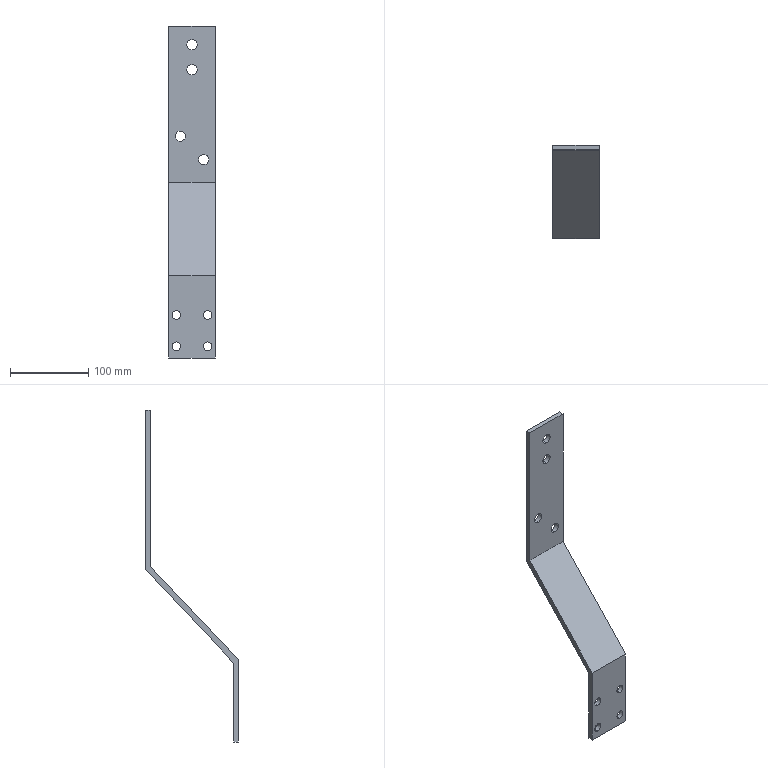Part | SolidWorks | features BaseBody 1 | 1 solid | 26 faces | box 60 x 119 x 425 mm | volume 174654 mm3 | cylinder 16 | plane 10 | commonest cylinder face diameters 11 x8 13 x8
STEP:
#1=CARTESIAN_POINT('',(546.946,-3258.473,957.471));
#2=VERTEX_POINT('',#1);
#3=CARTESIAN_POINT('',(546.946,-3258.473,944.471));
#4=VERTEX_POINT('',#3);
#5=CARTESIAN_POINT('',(546.946,-3258.473,950.971));
#6=DIRECTION('',(0.,-1.,0.));
#7=DIRECTION('',(0.,0.,-1.));
#8=AXIS2_PLACEMENT_3D('',#5,#6,#7);
#9=CIRCLE('',#8,6.5);
#10=EDGE_CURVE('',#2,#4,#9,.T.);
#11=ORIENTED_EDGE('',*,*,#10,.F.);
#12=CARTESIAN_POINT('',(546.946,-3264.473,957.471));
#13=VERTEX_POINT('',#12);
#14=CARTESIAN_POINT('',(546.946,-3307.534,957.471));
#15=DIRECTION('',(0.,-1.,0.));
#16=VECTOR('',#15,1000.);
#17=LINE('',#14,#16);
#18=EDGE_CURVE('',#2,#13,#17,.T.);
#19=ORIENTED_EDGE('',*,*,#18,.T.);
#20=CARTESIAN_POINT('',(546.946,-3264.473,944.471));
#21=VERTEX_POINT('',#20);
#22=CARTESIAN_POINT('',(546.946,-3264.473,950.971));
#23=DIRECTION('',(0.,1.,0.));
#24=DIRECTION('',(0.,0.,-1.));
#25=AXIS2_PLACEMENT_3D('',#22,#23,#24);
#26=CIRCLE('',#25,6.5);
#27=EDGE_CURVE('',#21,#13,#26,.T.);
#28=ORIENTED_EDGE('',*,*,#27,.F.);
#29=CARTESIAN_POINT('',(546.946,-3307.534,944.471));
#30=DIRECTION('',(0.,-1.,0.));
#31=VECTOR('',#30,1000.);
#32=LINE('',#29,#31);
#33=EDGE_CURVE('',#4,#21,#32,.T.);
#34=ORIENTED_EDGE('',*,*,#33,.F.);
#35=EDGE_LOOP('',(#11,#19,#28,#34));
#36=FACE_OUTER_BOUND('',#35,.T.);
#37=CARTESIAN_POINT('',(546.946,-3307.534,950.971));
#38=DIRECTION('',(0.,-1.,0.));
#39=DIRECTION('',(0.,0.,-1.));
#40=AXIS2_PLACEMENT_3D('',#37,#38,#39);
#41=CYLINDRICAL_SURFACE('',#40,6.5);
#42=ADVANCED_FACE('',(#36),#41,.F.);
#43=CARTESIAN_POINT('',(546.946,-3258.473,925.471));
#44=VERTEX_POINT('',#43);
#45=CARTESIAN_POINT('',(546.946,-3258.473,912.471));
#46=VERTEX_POINT('',#45);
#47=CARTESIAN_POINT('',(546.946,-3258.473,918.971));
#48=DIRECTION('',(0.,-1.,0.));
#49=DIRECTION('',(0.,0.,-1.));
#50=AXIS2_PLACEMENT_3D('',#47,#48,#49);
#51=CIRCLE('',#50,6.5);
#52=EDGE_CURVE('',#44,#46,#51,.T.);
#53=ORIENTED_EDGE('',*,*,#52,.F.);
#54=CARTESIAN_POINT('',(546.946,-3264.473,925.471));
#55=VERTEX_POINT('',#54);
#56=CARTESIAN_POINT('',(546.946,-3307.534,925.471));
#57=DIRECTION('',(0.,-1.,0.));
#58=VECTOR('',#57,1000.);
#59=LINE('',#56,#58);
#60=EDGE_CURVE('',#44,#55,#59,.T.);
#61=ORIENTED_EDGE('',*,*,#60,.T.);
#62=CARTESIAN_POINT('',(546.946,-3264.473,912.471));
#63=VERTEX_POINT('',#62);
#64=CARTESIAN_POINT('',(546.946,-3264.473,918.971));
#65=DIRECTION('',(0.,1.,0.));
#66=DIRECTION('',(0.,0.,-1.));
#67=AXIS2_PLACEMENT_3D('',#64,#65,#66);
#68=CIRCLE('',#67,6.5);
#69=EDGE_CURVE('',#63,#55,#68,.T.);
#70=ORIENTED_EDGE('',*,*,#69,.F.);
#71=CARTESIAN_POINT('',(546.946,-3307.534,912.471));
#72=DIRECTION('',(0.,-1.,0.));
#73=VECTOR('',#72,1000.);
#74=LINE('',#71,#73);
#75=EDGE_CURVE('',#46,#63,#74,.T.);
#76=ORIENTED_EDGE('',*,*,#75,.F.);
#77=EDGE_LOOP('',(#53,#61,#70,#76));
#78=FACE_OUTER_BOUND('',#77,.T.);
#79=CARTESIAN_POINT('',(546.946,-3307.534,918.971));
#80=DIRECTION('',(0.,-1.,0.));
#81=DIRECTION('',(0.,0.,-1.));
#82=AXIS2_PLACEMENT_3D('',#79,#80,#81);
#83=CYLINDRICAL_SURFACE('',#82,6.5);
#84=ADVANCED_FACE('',(#78),#83,.F.);
#85=CARTESIAN_POINT('',(531.946,-3258.473,840.471));
#86=VERTEX_POINT('',#85);
#87=CARTESIAN_POINT('',(531.946,-3258.473,827.471));
#88=VERTEX_POINT('',#87);
#89=CARTESIAN_POINT('',(531.946,-3258.473,833.971));
#90=DIRECTION('',(0.,-1.,0.));
#91=DIRECTION('',(0.,0.,-1.));
#92=AXIS2_PLACEMENT_3D('',#89,#90,#91);
#93=CIRCLE('',#92,6.5);
#94=EDGE_CURVE('',#86,#88,#93,.T.);
#95=ORIENTED_EDGE('',*,*,#94,.F.);
#96=CARTESIAN_POINT('',(531.946,-3264.473,840.471));
#97=VERTEX_POINT('',#96);
#98=CARTESIAN_POINT('',(531.946,-3298.213,840.471));
#99=DIRECTION('',(0.,-1.,0.));
#100=VECTOR('',#99,1000.);
#101=LINE('',#98,#100);
#102=EDGE_CURVE('',#86,#97,#101,.T.);
#103=ORIENTED_EDGE('',*,*,#102,.T.);
#104=CARTESIAN_POINT('',(531.946,-3264.473,827.471));
#105=VERTEX_POINT('',#104);
#106=CARTESIAN_POINT('',(531.946,-3264.473,833.971));
#107=DIRECTION('',(0.,1.,0.));
#108=DIRECTION('',(0.,0.,-1.));
#109=AXIS2_PLACEMENT_3D('',#106,#107,#108);
#110=CIRCLE('',#109,6.5);
#111=EDGE_CURVE('',#105,#97,#110,.T.);
#112=ORIENTED_EDGE('',*,*,#111,.F.);
#113=CARTESIAN_POINT('',(531.946,-3298.213,827.471));
#114=DIRECTION('',(0.,-1.,0.));
#115=VECTOR('',#114,1000.);
#116=LINE('',#113,#115);
#117=EDGE_CURVE('',#88,#105,#116,.T.);
#118=ORIENTED_EDGE('',*,*,#117,.F.);
#119=EDGE_LOOP('',(#95,#103,#112,#118));
#120=FACE_OUTER_BOUND('',#119,.T.);
#121=CARTESIAN_POINT('',(531.946,-3298.213,833.971));
#122=DIRECTION('',(0.,-1.,0.));
#123=DIRECTION('',(0.,0.,-1.));
#124=AXIS2_PLACEMENT_3D('',#121,#122,#123);
#125=CYLINDRICAL_SURFACE('',#124,6.5);
#126=ADVANCED_FACE('',(#120),#125,.F.);
#127=CARTESIAN_POINT('',(561.946,-3258.473,810.471));
#128=VERTEX_POINT('',#127);
#129=CARTESIAN_POINT('',(561.946,-3258.473,797.471));
#130=VERTEX_POINT('',#129);
#131=CARTESIAN_POINT('',(561.946,-3258.473,803.971));
#132=DIRECTION('',(0.,-1.,0.));
#133=DIRECTION('',(0.,0.,-1.));
#134=AXIS2_PLACEMENT_3D('',#131,#132,#133);
#135=CIRCLE('',#134,6.5);
#136=EDGE_CURVE('',#128,#130,#135,.T.);
#137=ORIENTED_EDGE('',*,*,#136,.F.);
#138=CARTESIAN_POINT('',(561.946,-3264.473,810.471));
#139=VERTEX_POINT('',#138);
#140=CARTESIAN_POINT('',(561.946,-3242.254,810.471));
#141=DIRECTION('',(0.,-1.,0.));
#142=VECTOR('',#141,1000.);
#143=LINE('',#140,#142);
#144=EDGE_CURVE('',#128,#139,#143,.T.);
#145=ORIENTED_EDGE('',*,*,#144,.T.);
#146=CARTESIAN_POINT('',(561.946,-3264.473,797.471));
#147=VERTEX_POINT('',#146);
#148=CARTESIAN_POINT('',(561.946,-3264.473,803.971));
#149=DIRECTION('',(0.,1.,0.));
#150=DIRECTION('',(0.,0.,-1.));
#151=AXIS2_PLACEMENT_3D('',#148,#149,#150);
#152=CIRCLE('',#151,6.5);
#153=EDGE_CURVE('',#147,#139,#152,.T.);
#154=ORIENTED_EDGE('',*,*,#153,.F.);
#155=CARTESIAN_POINT('',(561.946,-3242.254,797.471));
#156=DIRECTION('',(0.,-1.,0.));
#157=VECTOR('',#156,1000.);
#158=LINE('',#155,#157);
#159=EDGE_CURVE('',#130,#147,#158,.T.);
#160=ORIENTED_EDGE('',*,*,#159,.F.);
#161=EDGE_LOOP('',(#137,#145,#154,#160));
#162=FACE_OUTER_BOUND('',#161,.T.);
#163=CARTESIAN_POINT('',(561.946,-3242.254,803.971));
#164=DIRECTION('',(0.,-1.,0.));
#165=DIRECTION('',(0.,0.,-1.));
#166=AXIS2_PLACEMENT_3D('',#163,#164,#165);
#167=CYLINDRICAL_SURFACE('',#166,6.5);
#168=ADVANCED_FACE('',(#162),#167,.F.);
#169=CARTESIAN_POINT('',(526.946,-3371.473,570.471));
#170=VERTEX_POINT('',#169);
#171=CARTESIAN_POINT('',(526.946,-3371.473,559.471));
#172=VERTEX_POINT('',#171);
#173=CARTESIAN_POINT('',(526.946,-3371.473,564.971));
#174=DIRECTION('',(0.,-1.,0.));
#175=DIRECTION('',(0.,0.,-1.));
#176=AXIS2_PLACEMENT_3D('',#173,#174,#175);
#177=CIRCLE('',#176,5.5);
#178=EDGE_CURVE('',#170,#172,#177,.T.);
#179=ORIENTED_EDGE('',*,*,#178,.F.);
#180=CARTESIAN_POINT('',(526.946,-3377.473,570.471));
#181=VERTEX_POINT('',#180);
#182=CARTESIAN_POINT('',(526.946,-3426.67,570.471));
#183=DIRECTION('',(0.,-1.,0.));
#184=VECTOR('',#183,1000.);
#185=LINE('',#182,#184);
#186=EDGE_CURVE('',#170,#181,#185,.T.);
#187=ORIENTED_EDGE('',*,*,#186,.T.);
#188=CARTESIAN_POINT('',(526.946,-3377.473,559.471));
#189=VERTEX_POINT('',#188);
#190=CARTESIAN_POINT('',(526.946,-3377.473,564.971));
#191=DIRECTION('',(0.,1.,0.));
#192=DIRECTION('',(0.,0.,-1.));
#193=AXIS2_PLACEMENT_3D('',#190,#191,#192);
#194=CIRCLE('',#193,5.5);
#195=EDGE_CURVE('',#189,#181,#194,.T.);
#196=ORIENTED_EDGE('',*,*,#195,.F.);
#197=CARTESIAN_POINT('',(526.946,-3426.67,559.471));
#198=DIRECTION('',(0.,-1.,0.));
#199=VECTOR('',#198,1000.);
#200=LINE('',#197,#199);
#201=EDGE_CURVE('',#172,#189,#200,.T.);
#202=ORIENTED_EDGE('',*,*,#201,.F.);
#203=EDGE_LOOP('',(#179,#187,#196,#202));
#204=FACE_OUTER_BOUND('',#203,.T.);
#205=CARTESIAN_POINT('',(526.946,-3426.67,564.971));
#206=DIRECTION('',(0.,-1.,0.));
#207=DIRECTION('',(0.,0.,-1.));
#208=AXIS2_PLACEMENT_3D('',#205,#206,#207);
#209=CYLINDRICAL_SURFACE('',#208,5.5);
#210=ADVANCED_FACE('',(#204),#209,.F.);
#211=CARTESIAN_POINT('',(526.946,-3371.473,610.471));
#212=VERTEX_POINT('',#211);
#213=CARTESIAN_POINT('',(526.946,-3371.473,599.471));
#214=VERTEX_POINT('',#213);
#215=CARTESIAN_POINT('',(526.946,-3371.473,604.971));
#216=DIRECTION('',(0.,-1.,0.));
#217=DIRECTION('',(0.,0.,-1.));
#218=AXIS2_PLACEMENT_3D('',#215,#216,#217);
#219=CIRCLE('',#218,5.5);
#220=EDGE_CURVE('',#212,#214,#219,.T.);
#221=ORIENTED_EDGE('',*,*,#220,.F.);
#222=CARTESIAN_POINT('',(526.946,-3377.473,610.471));
#223=VERTEX_POINT('',#222);
#224=CARTESIAN_POINT('',(526.946,-3426.67,610.471));
#225=DIRECTION('',(0.,-1.,0.));
#226=VECTOR('',#225,1000.);
#227=LINE('',#224,#226);
#228=EDGE_CURVE('',#212,#223,#227,.T.);
#229=ORIENTED_EDGE('',*,*,#228,.T.);
#230=CARTESIAN_POINT('',(526.946,-3377.473,599.471));
#231=VERTEX_POINT('',#230);
#232=CARTESIAN_POINT('',(526.946,-3377.473,604.971));
#233=DIRECTION('',(0.,1.,0.));
#234=DIRECTION('',(0.,0.,-1.));
#235=AXIS2_PLACEMENT_3D('',#232,#233,#234);
#236=CIRCLE('',#235,5.5);
#237=EDGE_CURVE('',#231,#223,#236,.T.);
#238=ORIENTED_EDGE('',*,*,#237,.F.);
#239=CARTESIAN_POINT('',(526.946,-3426.67,599.471));
#240=DIRECTION('',(0.,-1.,0.));
#241=VECTOR('',#240,1000.);
#242=LINE('',#239,#241);
#243=EDGE_CURVE('',#214,#231,#242,.T.);
#244=ORIENTED_EDGE('',*,*,#243,.F.);
#245=EDGE_LOOP('',(#221,#229,#238,#244));
#246=FACE_OUTER_BOUND('',#245,.T.);
#247=CARTESIAN_POINT('',(526.946,-3426.67,604.971));
#248=DIRECTION('',(0.,-1.,0.));
#249=DIRECTION('',(0.,0.,-1.));
#250=AXIS2_PLACEMENT_3D('',#247,#248,#249);
#251=CYLINDRICAL_SURFACE('',#250,5.5);
#252=ADVANCED_FACE('',(#246),#251,.F.);
#253=CARTESIAN_POINT('',(566.946,-3377.473,599.471));
#254=VERTEX_POINT('',#253);
#255=CARTESIAN_POINT('',(566.946,-3377.473,610.471));
#256=VERTEX_POINT('',#255);
#257=CARTESIAN_POINT('',(566.946,-3377.473,604.971));
#258=DIRECTION('',(0.,1.,0.));
#259=DIRECTION('',(0.,0.,1.));
#260=AXIS2_PLACEMENT_3D('',#257,#258,#259);
#261=CIRCLE('',#260,5.5);
#262=EDGE_CURVE('',#254,#256,#261,.T.);
#263=ORIENTED_EDGE('',*,*,#262,.F.);
#264=CARTESIAN_POINT('',(566.946,-3371.473,599.471));
#265=VERTEX_POINT('',#264);
#266=CARTESIAN_POINT('',(566.946,-3426.67,599.471));
#267=DIRECTION('',(0.,1.,0.));
#268=VECTOR('',#267,1000.);
#269=LINE('',#266,#268);
#270=EDGE_CURVE('',#254,#265,#269,.T.);
#271=ORIENTED_EDGE('',*,*,#270,.T.);
#272=CARTESIAN_POINT('',(566.946,-3371.473,610.471));
#273=VERTEX_POINT('',#272);
#274=CARTESIAN_POINT('',(566.946,-3371.473,604.971));
#275=DIRECTION('',(0.,-1.,0.));
#276=DIRECTION('',(0.,0.,1.));
#277=AXIS2_PLACEMENT_3D('',#274,#275,#276);
#278=CIRCLE('',#277,5.5);
#279=EDGE_CURVE('',#273,#265,#278,.T.);
#280=ORIENTED_EDGE('',*,*,#279,.F.);
#281=CARTESIAN_POINT('',(566.946,-3426.67,610.471));
#282=DIRECTION('',(0.,1.,0.));
#283=VECTOR('',#282,1000.);
#284=LINE('',#281,#283);
#285=EDGE_CURVE('',#256,#273,#284,.T.);
#286=ORIENTED_EDGE('',*,*,#285,.F.);
#287=EDGE_LOOP('',(#263,#271,#280,#286));
#288=FACE_OUTER_BOUND('',#287,.T.);
#289=CARTESIAN_POINT('',(566.946,-3426.67,604.971));
#290=DIRECTION('',(0.,1.,0.));
#291=DIRECTION('',(0.,0.,1.));
#292=AXIS2_PLACEMENT_3D('',#289,#290,#291);
#293=CYLINDRICAL_SURFACE('',#292,5.5);
#294=ADVANCED_FACE('',(#288),#293,.F.);
#295=CARTESIAN_POINT('',(566.946,-3377.473,559.471));
#296=VERTEX_POINT('',#295);
#297=CARTESIAN_POINT('',(566.946,-3377.473,570.471));
#298=VERTEX_POINT('',#297);
#299=CARTESIAN_POINT('',(566.946,-3377.473,564.971));
#300=DIRECTION('',(0.,1.,0.));
#301=DIRECTION('',(0.,0.,1.));
#302=AXIS2_PLACEMENT_3D('',#299,#300,#301);
#303=CIRCLE('',#302,5.5);
#304=EDGE_CURVE('',#296,#298,#303,.T.);
#305=ORIENTED_EDGE('',*,*,#304,.F.);
#306=CARTESIAN_POINT('',(566.946,-3371.473,559.471));
#307=VERTEX_POINT('',#306);
#308=CARTESIAN_POINT('',(566.946,-3426.67,559.471));
#309=DIRECTION('',(0.,1.,0.));
#310=VECTOR('',#309,1000.);
#311=LINE('',#308,#310);
#312=EDGE_CURVE('',#296,#307,#311,.T.);
#313=ORIENTED_EDGE('',*,*,#312,.T.);
#314=CARTESIAN_POINT('',(566.946,-3371.473,570.471));
#315=VERTEX_POINT('',#314);
#316=CARTESIAN_POINT('',(566.946,-3371.473,564.971));
#317=DIRECTION('',(0.,-1.,0.));
#318=DIRECTION('',(0.,0.,1.));
#319=AXIS2_PLACEMENT_3D('',#316,#317,#318);
#320=CIRCLE('',#319,5.5);
#321=EDGE_CURVE('',#315,#307,#320,.T.);
#322=ORIENTED_EDGE('',*,*,#321,.F.);
#323=CARTESIAN_POINT('',(566.946,-3426.67,570.471));
#324=DIRECTION('',(0.,1.,0.));
#325=VECTOR('',#324,1000.);
#326=LINE('',#323,#325);
#327=EDGE_CURVE('',#298,#315,#326,.T.);
#328=ORIENTED_EDGE('',*,*,#327,.F.);
#329=EDGE_LOOP('',(#305,#313,#322,#328));
#330=FACE_OUTER_BOUND('',#329,.T.);
#331=CARTESIAN_POINT('',(566.946,-3426.67,564.971));
#332=DIRECTION('',(0.,1.,0.));
#333=DIRECTION('',(0.,0.,1.));
#334=AXIS2_PLACEMENT_3D('',#331,#332,#333);
#335=CYLINDRICAL_SURFACE('',#334,5.5);
#336=ADVANCED_FACE('',(#330),#335,.F.);
#337=CARTESIAN_POINT('',(576.946,-3258.473,974.971));
#338=VERTEX_POINT('',#337);
#339=CARTESIAN_POINT('',(576.946,-3258.473,770.971));
#340=VERTEX_POINT('',#339);
#341=CARTESIAN_POINT('',(576.946,-3258.473,790.971));
#342=DIRECTION('',(0.,0.,-1.));
#343=VECTOR('',#342,1000.);
#344=LINE('',#341,#343);
#345=EDGE_CURVE('',#338,#340,#344,.T.);
#346=ORIENTED_EDGE('',*,*,#345,.T.);
#347=CARTESIAN_POINT('',(516.946,-3258.473,770.971));
#348=VERTEX_POINT('',#347);
#349=CARTESIAN_POINT('',(576.946,-3258.473,770.971));
#350=DIRECTION('',(-1.,0.,0.));
#351=VECTOR('',#350,1000.);
#352=LINE('',#349,#351);
#353=EDGE_CURVE('',#340,#348,#352,.T.);
#354=ORIENTED_EDGE('',*,*,#353,.T.);
#355=CARTESIAN_POINT('',(516.946,-3258.473,974.971));
#356=VERTEX_POINT('',#355);
#357=CARTESIAN_POINT('',(516.946,-3258.473,790.971));
#358=DIRECTION('',(0.,0.,1.));
#359=VECTOR('',#358,1000.);
#360=LINE('',#357,#359);
#361=EDGE_CURVE('',#348,#356,#360,.T.);
#362=ORIENTED_EDGE('',*,*,#361,.T.);
#363=CARTESIAN_POINT('',(576.946,-3258.473,974.971));
#364=DIRECTION('',(1.,0.,0.));
#365=VECTOR('',#364,1000.);
#366=LINE('',#363,#365);
#367=EDGE_CURVE('',#356,#338,#366,.T.);
#368=ORIENTED_EDGE('',*,*,#367,.T.);
#369=EDGE_LOOP('',(#346,#354,#362,#368));
#370=FACE_OUTER_BOUND('',#369,.T.);
#371=CARTESIAN_POINT('',(546.946,-3258.473,950.971));
#372=DIRECTION('',(0.,-1.,0.));
#373=DIRECTION('',(0.,0.,-1.));
#374=AXIS2_PLACEMENT_3D('',#371,#372,#373);
#375=CIRCLE('',#374,6.5);
#376=EDGE_CURVE('',#4,#2,#375,.T.);
#377=ORIENTED_EDGE('',*,*,#376,.T.);
#378=ORIENTED_EDGE('',*,*,#10,.T.);
#379=EDGE_LOOP('',(#377,#378));
#380=FACE_BOUND('',#379,.T.);
#381=CARTESIAN_POINT('',(546.946,-3258.473,918.971));
#382=DIRECTION('',(0.,-1.,0.));
#383=DIRECTION('',(0.,0.,-1.));
#384=AXIS2_PLACEMENT_3D('',#381,#382,#383);
#385=CIRCLE('',#384,6.5);
#386=EDGE_CURVE('',#46,#44,#385,.T.);
#387=ORIENTED_EDGE('',*,*,#386,.T.);
#388=ORIENTED_EDGE('',*,*,#52,.T.);
#389=EDGE_LOOP('',(#387,#388));
#390=FACE_BOUND('',#389,.T.);
#391=CARTESIAN_POINT('',(531.946,-3258.473,833.971));
#392=DIRECTION('',(0.,-1.,0.));
#393=DIRECTION('',(0.,0.,-1.));
#394=AXIS2_PLACEMENT_3D('',#391,#392,#393);
#395=CIRCLE('',#394,6.5);
#396=EDGE_CURVE('',#88,#86,#395,.T.);
#397=ORIENTED_EDGE('',*,*,#396,.T.);
#398=ORIENTED_EDGE('',*,*,#94,.T.);
#399=EDGE_LOOP('',(#397,#398));
#400=FACE_BOUND('',#399,.T.);
#401=CARTESIAN_POINT('',(561.946,-3258.473,803.971));
#402=DIRECTION('',(0.,-1.,0.));
#403=DIRECTION('',(0.,0.,-1.));
#404=AXIS2_PLACEMENT_3D('',#401,#402,#403);
#405=CIRCLE('',#404,6.5);
#406=EDGE_CURVE('',#130,#128,#405,.T.);
#407=ORIENTED_EDGE('',*,*,#406,.T.);
#408=ORIENTED_EDGE('',*,*,#136,.T.);
#409=EDGE_LOOP('',(#407,#408));
#410=FACE_BOUND('',#409,.T.);
#411=CARTESIAN_POINT('',(576.946,-3258.473,790.971));
#412=DIRECTION('',(0.,1.,0.));
#413=DIRECTION('',(0.,0.,1.));
#414=AXIS2_PLACEMENT_3D('',#411,#412,#413);
#415=PLANE('',#414);
#416=ADVANCED_FACE('',(#370,#380,#390,#400,#410),#415,.T.);
#417=CARTESIAN_POINT('',(576.946,-3371.473,650.971));
#418=VERTEX_POINT('',#417);
#419=CARTESIAN_POINT('',(576.946,-3371.473,650.971));
#420=DIRECTION('',(0.,-0.6856,-0.728));
#421=VECTOR('',#420,1000.);
#422=LINE('',#419,#421);
#423=EDGE_CURVE('',#340,#418,#422,.T.);
#424=ORIENTED_EDGE('',*,*,#423,.T.);
#425=CARTESIAN_POINT('',(516.946,-3371.473,650.971));
#426=VERTEX_POINT('',#425);
#427=CARTESIAN_POINT('',(576.946,-3371.473,650.971));
#428=DIRECTION('',(-1.,0.,0.));
#429=VECTOR('',#428,1000.);
#430=LINE('',#427,#429);
#431=EDGE_CURVE('',#418,#426,#430,.T.);
#432=ORIENTED_EDGE('',*,*,#431,.T.);
#433=CARTESIAN_POINT('',(516.946,-3371.473,650.971));
#434=DIRECTION('',(0.,0.6856,0.728));
#435=VECTOR('',#434,1000.);
#436=LINE('',#433,#435);
#437=EDGE_CURVE('',#426,#348,#436,.T.);
#438=ORIENTED_EDGE('',*,*,#437,.T.);
#439=ORIENTED_EDGE('',*,*,#353,.F.);
#440=EDGE_LOOP('',(#424,#432,#438,#439));
#441=FACE_OUTER_BOUND('',#440,.T.);
#442=CARTESIAN_POINT('',(576.946,-3371.473,650.971));
#443=DIRECTION('',(0.,0.728,-0.6856));
#444=DIRECTION('',(0.,0.6856,0.728));
#445=AXIS2_PLACEMENT_3D('',#442,#443,#444);
#446=PLANE('',#445);
#447=ADVANCED_FACE('',(#441),#446,.T.);
#448=CARTESIAN_POINT('',(576.946,-3264.473,774.971));
#449=VERTEX_POINT('',#448);
#450=CARTESIAN_POINT('',(576.946,-3377.473,654.971));
#451=VERTEX_POINT('',#450);
#452=CARTESIAN_POINT('',(576.946,-3264.473,774.971));
#453=DIRECTION('',(0.,-0.6856,-0.728));
#454=VECTOR('',#453,1000.);
#455=LINE('',#452,#454);
#456=EDGE_CURVE('',#449,#451,#455,.T.);
#457=ORIENTED_EDGE('',*,*,#456,.T.);
#458=CARTESIAN_POINT('',(576.946,-3377.473,549.971));
#459=VERTEX_POINT('',#458);
#460=CARTESIAN_POINT('',(576.946,-3377.473,759.692));
#461=DIRECTION('',(0.,0.,-1.));
#462=VECTOR('',#461,1000.);
#463=LINE('',#460,#462);
#464=EDGE_CURVE('',#451,#459,#463,.T.);
#465=ORIENTED_EDGE('',*,*,#464,.T.);
#466=CARTESIAN_POINT('',(576.946,-3371.473,549.971));
#467=VERTEX_POINT('',#466);
#468=CARTESIAN_POINT('',(576.946,-3310.967,549.971));
#469=DIRECTION('',(0.,1.,0.));
#470=VECTOR('',#469,1000.);
#471=LINE('',#468,#470);
#472=EDGE_CURVE('',#459,#467,#471,.T.);
#473=ORIENTED_EDGE('',*,*,#472,.T.);
#474=CARTESIAN_POINT('',(576.946,-3371.473,759.692));
#475=DIRECTION('',(0.,0.,1.));
#476=VECTOR('',#475,1000.);
#477=LINE('',#474,#476);
#478=EDGE_CURVE('',#467,#418,#477,.T.);
#479=ORIENTED_EDGE('',*,*,#478,.T.);
#480=ORIENTED_EDGE('',*,*,#423,.F.);
#481=ORIENTED_EDGE('',*,*,#345,.F.);
#482=CARTESIAN_POINT('',(576.946,-3264.473,974.971));
#483=VERTEX_POINT('',#482);
#484=CARTESIAN_POINT('',(576.946,-3310.967,974.971));
#485=DIRECTION('',(0.,-1.,0.));
#486=VECTOR('',#485,1000.);
#487=LINE('',#484,#486);
#488=EDGE_CURVE('',#338,#483,#487,.T.);
#489=ORIENTED_EDGE('',*,*,#488,.T.);
#490=CARTESIAN_POINT('',(576.946,-3264.473,759.692));
#491=DIRECTION('',(0.,0.,-1.));
#492=VECTOR('',#491,1000.);
#493=LINE('',#490,#492);
#494=EDGE_CURVE('',#483,#449,#493,.T.);
#495=ORIENTED_EDGE('',*,*,#494,.T.);
#496=EDGE_LOOP('',(#457,#465,#473,#479,#480,#481,#489,#495));
#497=FACE_OUTER_BOUND('',#496,.T.);
#498=CARTESIAN_POINT('',(576.946,-3310.967,759.692));
#499=DIRECTION('',(1.,0.,0.));
#500=DIRECTION('',(0.,0.,-1.));
#501=AXIS2_PLACEMENT_3D('',#498,#499,#500);
#502=PLANE('',#501);
#503=ADVANCED_FACE('',(#497),#502,.T.);
#504=ORIENTED_EDGE('',*,*,#488,.F.);
#505=ORIENTED_EDGE('',*,*,#367,.F.);
#506=CARTESIAN_POINT('',(516.946,-3264.473,974.971));
#507=VERTEX_POINT('',#506);
#508=CARTESIAN_POINT('',(516.946,-3258.473,974.971));
#509=DIRECTION('',(0.,-1.,0.));
#510=VECTOR('',#509,1000.);
#511=LINE('',#508,#510);
#512=EDGE_CURVE('',#356,#507,#511,.T.);
#513=ORIENTED_EDGE('',*,*,#512,.T.);
#514=CARTESIAN_POINT('',(576.946,-3264.473,974.971));
#515=DIRECTION('',(1.,0.,0.));
#516=VECTOR('',#515,1000.);
#517=LINE('',#514,#516);
#518=EDGE_CURVE('',#507,#483,#517,.T.);
#519=ORIENTED_EDGE('',*,*,#518,.T.);
#520=EDGE_LOOP('',(#504,#505,#513,#519));
#521=FACE_OUTER_BOUND('',#520,.T.);
#522=CARTESIAN_POINT('',(576.946,-3258.473,974.971));
#523=DIRECTION('',(0.,0.,1.));
#524=DIRECTION('',(1.,0.,0.));
#525=AXIS2_PLACEMENT_3D('',#522,#523,#524);
#526=PLANE('',#525);
#527=ADVANCED_FACE('',(#521),#526,.T.);
#528=CARTESIAN_POINT('',(516.946,-3377.473,549.971));
#529=VERTEX_POINT('',#528);
#530=CARTESIAN_POINT('',(516.946,-3371.473,549.971));
#531=VERTEX_POINT('',#530);
#532=CARTESIAN_POINT('',(516.946,-3310.967,549.971));
#533=DIRECTION('',(0.,1.,0.));
#534=VECTOR('',#533,1000.);
#535=LINE('',#532,#534);
#536=EDGE_CURVE('',#529,#531,#535,.T.);
#537=ORIENTED_EDGE('',*,*,#536,.F.);
#538=CARTESIAN_POINT('',(516.946,-3377.473,654.971));
#539=VERTEX_POINT('',#538);
#540=CARTESIAN_POINT('',(516.946,-3377.473,739.692));
#541=DIRECTION('',(0.,0.,-1.));
#542=VECTOR('',#541,1000.);
#543=LINE('',#540,#542);
#544=EDGE_CURVE('',#539,#529,#543,.T.);
#545=ORIENTED_EDGE('',*,*,#544,.F.);
#546=CARTESIAN_POINT('',(516.946,-3264.473,774.971));
#547=VERTEX_POINT('',#546);
#548=CARTESIAN_POINT('',(516.946,-3264.473,774.971));
#549=DIRECTION('',(0.,-0.6856,-0.728));
#550=VECTOR('',#549,1000.);
#551=LINE('',#548,#550);
#552=EDGE_CURVE('',#547,#539,#551,.T.);
#553=ORIENTED_EDGE('',*,*,#552,.F.);
#554=CARTESIAN_POINT('',(516.946,-3264.473,739.692));
#555=DIRECTION('',(0.,0.,-1.));
#556=VECTOR('',#555,1000.);
#557=LINE('',#554,#556);
#558=EDGE_CURVE('',#507,#547,#557,.T.);
#559=ORIENTED_EDGE('',*,*,#558,.F.);
#560=ORIENTED_EDGE('',*,*,#512,.F.);
#561=ORIENTED_EDGE('',*,*,#361,.F.);
#562=ORIENTED_EDGE('',*,*,#437,.F.);
#563=CARTESIAN_POINT('',(516.946,-3371.473,739.692));
#564=DIRECTION('',(0.,0.,1.));
#565=VECTOR('',#564,1000.);
#566=LINE('',#563,#565);
#567=EDGE_CURVE('',#531,#426,#566,.T.);
#568=ORIENTED_EDGE('',*,*,#567,.F.);
#569=EDGE_LOOP('',(#537,#545,#553,#559,#560,#561,#562,#568));
#570=FACE_OUTER_BOUND('',#569,.T.);
#571=CARTESIAN_POINT('',(516.946,-3310.967,739.692));
#572=DIRECTION('',(1.,0.,0.));
#573=DIRECTION('',(0.,0.,-1.));
#574=AXIS2_PLACEMENT_3D('',#571,#572,#573);
#575=PLANE('',#574);
#576=ADVANCED_FACE('',(#570),#575,.F.);
#577=ORIENTED_EDGE('',*,*,#18,.F.);
#578=ORIENTED_EDGE('',*,*,#376,.F.);
#579=ORIENTED_EDGE('',*,*,#33,.T.);
#580=CARTESIAN_POINT('',(546.946,-3264.473,950.971));
#581=DIRECTION('',(0.,1.,0.));
#582=DIRECTION('',(0.,0.,-1.));
#583=AXIS2_PLACEMENT_3D('',#580,#581,#582);
#584=CIRCLE('',#583,6.5);
#585=EDGE_CURVE('',#13,#21,#584,.T.);
#586=ORIENTED_EDGE('',*,*,#585,.F.);
#587=EDGE_LOOP('',(#577,#578,#579,#586));
#588=FACE_OUTER_BOUND('',#587,.T.);
#589=CARTESIAN_POINT('',(546.946,-3307.534,950.971));
#590=DIRECTION('',(0.,-1.,0.));
#591=DIRECTION('',(0.,0.,-1.));
#592=AXIS2_PLACEMENT_3D('',#589,#590,#591);
#593=CYLINDRICAL_SURFACE('',#592,6.5);
#594=ADVANCED_FACE('',(#588),#593,.F.);
#595=ORIENTED_EDGE('',*,*,#60,.F.);
#596=ORIENTED_EDGE('',*,*,#386,.F.);
#597=ORIENTED_EDGE('',*,*,#75,.T.);
#598=CARTESIAN_POINT('',(546.946,-3264.473,918.971));
#599=DIRECTION('',(0.,1.,0.));
#600=DIRECTION('',(0.,0.,-1.));
#601=AXIS2_PLACEMENT_3D('',#598,#599,#600);
#602=CIRCLE('',#601,6.5);
#603=EDGE_CURVE('',#55,#63,#602,.T.);
#604=ORIENTED_EDGE('',*,*,#603,.F.);
#605=EDGE_LOOP('',(#595,#596,#597,#604));
#606=FACE_OUTER_BOUND('',#605,.T.);
#607=CARTESIAN_POINT('',(546.946,-3307.534,918.971));
#608=DIRECTION('',(0.,-1.,0.));
#609=DIRECTION('',(0.,0.,-1.));
#610=AXIS2_PLACEMENT_3D('',#607,#608,#609);
#611=CYLINDRICAL_SURFACE('',#610,6.5);
#612=ADVANCED_FACE('',(#606),#611,.F.);
#613=ORIENTED_EDGE('',*,*,#102,.F.);
#614=ORIENTED_EDGE('',*,*,#396,.F.);
#615=ORIENTED_EDGE('',*,*,#117,.T.);
#616=CARTESIAN_POINT('',(531.946,-3264.473,833.971));
#617=DIRECTION('',(0.,1.,0.));
#618=DIRECTION('',(0.,0.,-1.));
#619=AXIS2_PLACEMENT_3D('',#616,#617,#618);
#620=CIRCLE('',#619,6.5);
#621=EDGE_CURVE('',#97,#105,#620,.T.);
#622=ORIENTED_EDGE('',*,*,#621,.F.);
#623=EDGE_LOOP('',(#613,#614,#615,#622));
#624=FACE_OUTER_BOUND('',#623,.T.);
#625=CARTESIAN_POINT('',(531.946,-3298.213,833.971));
#626=DIRECTION('',(0.,-1.,0.));
#627=DIRECTION('',(0.,0.,-1.));
#628=AXIS2_PLACEMENT_3D('',#625,#626,#627);
#629=CYLINDRICAL_SURFACE('',#628,6.5);
#630=ADVANCED_FACE('',(#624),#629,.F.);
#631=ORIENTED_EDGE('',*,*,#144,.F.);
#632=ORIENTED_EDGE('',*,*,#406,.F.);
#633=ORIENTED_EDGE('',*,*,#159,.T.);
#634=CARTESIAN_POINT('',(561.946,-3264.473,803.971));
#635=DIRECTION('',(0.,1.,0.));
#636=DIRECTION('',(0.,0.,-1.));
#637=AXIS2_PLACEMENT_3D('',#634,#635,#636);
#638=CIRCLE('',#637,6.5);
#639=EDGE_CURVE('',#139,#147,#638,.T.);
#640=ORIENTED_EDGE('',*,*,#639,.F.);
#641=EDGE_LOOP('',(#631,#632,#633,#640));
#642=FACE_OUTER_BOUND('',#641,.T.);
#643=CARTESIAN_POINT('',(561.946,-3242.254,803.971));
#644=DIRECTION('',(0.,-1.,0.));
#645=DIRECTION('',(0.,0.,-1.));
#646=AXIS2_PLACEMENT_3D('',#643,#644,#645);
#647=CYLINDRICAL_SURFACE('',#646,6.5);
#648=ADVANCED_FACE('',(#642),#647,.F.);
#649=ORIENTED_EDGE('',*,*,#478,.F.);
#650=CARTESIAN_POINT('',(576.946,-3371.473,549.971));
#651=DIRECTION('',(-1.,0.,0.));
#652=VECTOR('',#651,1000.);
#653=LINE('',#650,#652);
#654=EDGE_CURVE('',#467,#531,#653,.T.);
#655=ORIENTED_EDGE('',*,*,#654,.T.);
#656=ORIENTED_EDGE('',*,*,#567,.T.);
#657=ORIENTED_EDGE('',*,*,#431,.F.);
#658=EDGE_LOOP('',(#649,#655,#656,#657));
#659=FACE_OUTER_BOUND('',#658,.T.);
#660=CARTESIAN_POINT('',(526.946,-3371.473,564.971));
#661=DIRECTION('',(0.,-1.,0.));
#662=DIRECTION('',(0.,0.,-1.));
#663=AXIS2_PLACEMENT_3D('',#660,#661,#662);
#664=CIRCLE('',#663,5.5);
#665=EDGE_CURVE('',#172,#170,#664,.T.);
#666=ORIENTED_EDGE('',*,*,#665,.T.);
#667=ORIENTED_EDGE('',*,*,#178,.T.);
#668=EDGE_LOOP('',(#666,#667));
#669=FACE_BOUND('',#668,.T.);
#670=CARTESIAN_POINT('',(526.946,-3371.473,604.971));
#671=DIRECTION('',(0.,-1.,0.));
#672=DIRECTION('',(0.,0.,-1.));
#673=AXIS2_PLACEMENT_3D('',#670,#671,#672);
#674=CIRCLE('',#673,5.5);
#675=EDGE_CURVE('',#214,#212,#674,.T.);
#676=ORIENTED_EDGE('',*,*,#675,.T.);
#677=ORIENTED_EDGE('',*,*,#220,.T.);
#678=EDGE_LOOP('',(#676,#677));
#679=FACE_BOUND('',#678,.T.);
#680=ORIENTED_EDGE('',*,*,#279,.T.);
#681=CARTESIAN_POINT('',(566.946,-3371.473,604.971));
#682=DIRECTION('',(0.,-1.,0.));
#683=DIRECTION('',(0.,0.,1.));
#684=AXIS2_PLACEMENT_3D('',#681,#682,#683);
#685=CIRCLE('',#684,5.5);
#686=EDGE_CURVE('',#265,#273,#685,.T.);
#687=ORIENTED_EDGE('',*,*,#686,.T.);
#688=EDGE_LOOP('',(#680,#687));
#689=FACE_BOUND('',#688,.T.);
#690=ORIENTED_EDGE('',*,*,#321,.T.);
#691=CARTESIAN_POINT('',(566.946,-3371.473,564.971));
#692=DIRECTION('',(0.,-1.,0.));
#693=DIRECTION('',(0.,0.,1.));
#694=AXIS2_PLACEMENT_3D('',#691,#692,#693);
#695=CIRCLE('',#694,5.5);
#696=EDGE_CURVE('',#307,#315,#695,.T.);
#697=ORIENTED_EDGE('',*,*,#696,.T.);
#698=EDGE_LOOP('',(#690,#697));
#699=FACE_BOUND('',#698,.T.);
#700=CARTESIAN_POINT('',(576.946,-3371.473,549.971));
#701=DIRECTION('',(0.,1.,0.));
#702=DIRECTION('',(0.,0.,1.));
#703=AXIS2_PLACEMENT_3D('',#700,#701,#702);
#704=PLANE('',#703);
#705=ADVANCED_FACE('',(#659,#669,#679,#689,#699),#704,.T.);
#706=ORIENTED_EDGE('',*,*,#464,.F.);
#707=CARTESIAN_POINT('',(576.946,-3377.473,654.971));
#708=DIRECTION('',(-1.,0.,0.));
#709=VECTOR('',#708,1000.);
#710=LINE('',#707,#709);
#711=EDGE_CURVE('',#451,#539,#710,.T.);
#712=ORIENTED_EDGE('',*,*,#711,.T.);
#713=ORIENTED_EDGE('',*,*,#544,.T.);
#714=CARTESIAN_POINT('',(576.946,-3377.473,549.971));
#715=DIRECTION('',(1.,0.,0.));
#716=VECTOR('',#715,1000.);
#717=LINE('',#714,#716);
#718=EDGE_CURVE('',#529,#459,#717,.T.);
#719=ORIENTED_EDGE('',*,*,#718,.T.);
#720=EDGE_LOOP('',(#706,#712,#713,#719));
#721=FACE_OUTER_BOUND('',#720,.T.);
#722=ORIENTED_EDGE('',*,*,#195,.T.);
#723=CARTESIAN_POINT('',(526.946,-3377.473,564.971));
#724=DIRECTION('',(0.,1.,0.));
#725=DIRECTION('',(0.,0.,-1.));
#726=AXIS2_PLACEMENT_3D('',#723,#724,#725);
#727=CIRCLE('',#726,5.5);
#728=EDGE_CURVE('',#181,#189,#727,.T.);
#729=ORIENTED_EDGE('',*,*,#728,.T.);
#730=EDGE_LOOP('',(#722,#729));
#731=FACE_BOUND('',#730,.T.);
#732=ORIENTED_EDGE('',*,*,#237,.T.);
#733=CARTESIAN_POINT('',(526.946,-3377.473,604.971));
#734=DIRECTION('',(0.,1.,0.));
#735=DIRECTION('',(0.,0.,-1.));
#736=AXIS2_PLACEMENT_3D('',#733,#734,#735);
#737=CIRCLE('',#736,5.5);
#738=EDGE_CURVE('',#223,#231,#737,.T.);
#739=ORIENTED_EDGE('',*,*,#738,.T.);
#740=EDGE_LOOP('',(#732,#739));
#741=FACE_BOUND('',#740,.T.);
#742=CARTESIAN_POINT('',(566.946,-3377.473,604.971));
#743=DIRECTION('',(0.,1.,0.));
#744=DIRECTION('',(0.,0.,1.));
#745=AXIS2_PLACEMENT_3D('',#742,#743,#744);
#746=CIRCLE('',#745,5.5);
#747=EDGE_CURVE('',#256,#254,#746,.T.);
#748=ORIENTED_EDGE('',*,*,#747,.T.);
#749=ORIENTED_EDGE('',*,*,#262,.T.);
#750=EDGE_LOOP('',(#748,#749));
#751=FACE_BOUND('',#750,.T.);
#752=CARTESIAN_POINT('',(566.946,-3377.473,564.971));
#753=DIRECTION('',(0.,1.,0.));
#754=DIRECTION('',(0.,0.,1.));
#755=AXIS2_PLACEMENT_3D('',#752,#753,#754);
#756=CIRCLE('',#755,5.5);
#757=EDGE_CURVE('',#298,#296,#756,.T.);
#758=ORIENTED_EDGE('',*,*,#757,.T.);
#759=ORIENTED_EDGE('',*,*,#304,.T.);
#760=EDGE_LOOP('',(#758,#759));
#761=FACE_BOUND('',#760,.T.);
#762=CARTESIAN_POINT('',(576.946,-3377.473,654.971));
#763=DIRECTION('',(0.,-1.,0.));
#764=DIRECTION('',(0.,0.,-1.));
#765=AXIS2_PLACEMENT_3D('',#762,#763,#764);
#766=PLANE('',#765);
#767=ADVANCED_FACE('',(#721,#731,#741,#751,#761),#766,.T.);
#768=ORIENTED_EDGE('',*,*,#456,.F.);
#769=CARTESIAN_POINT('',(576.946,-3264.473,774.971));
#770=DIRECTION('',(-1.,0.,0.));
#771=VECTOR('',#770,1000.);
#772=LINE('',#769,#771);
#773=EDGE_CURVE('',#449,#547,#772,.T.);
#774=ORIENTED_EDGE('',*,*,#773,.T.);
#775=ORIENTED_EDGE('',*,*,#552,.T.);
#776=ORIENTED_EDGE('',*,*,#711,.F.);
#777=EDGE_LOOP('',(#768,#774,#775,#776));
#778=FACE_OUTER_BOUND('',#777,.T.);
#779=CARTESIAN_POINT('',(576.946,-3264.473,774.971));
#780=DIRECTION('',(0.,-0.728,0.6856));
#781=DIRECTION('',(0.,-0.6856,-0.728));
#782=AXIS2_PLACEMENT_3D('',#779,#780,#781);
#783=PLANE('',#782);
#784=ADVANCED_FACE('',(#778),#783,.T.);
#785=ORIENTED_EDGE('',*,*,#494,.F.);
#786=ORIENTED_EDGE('',*,*,#518,.F.);
#787=ORIENTED_EDGE('',*,*,#558,.T.);
#788=ORIENTED_EDGE('',*,*,#773,.F.);
#789=EDGE_LOOP('',(#785,#786,#787,#788));
#790=FACE_OUTER_BOUND('',#789,.T.);
#791=ORIENTED_EDGE('',*,*,#27,.T.);
#792=ORIENTED_EDGE('',*,*,#585,.T.);
#793=EDGE_LOOP('',(#791,#792));
#794=FACE_BOUND('',#793,.T.);
#795=ORIENTED_EDGE('',*,*,#69,.T.);
#796=ORIENTED_EDGE('',*,*,#603,.T.);
#797=EDGE_LOOP('',(#795,#796));
#798=FACE_BOUND('',#797,.T.);
#799=ORIENTED_EDGE('',*,*,#111,.T.);
#800=ORIENTED_EDGE('',*,*,#621,.T.);
#801=EDGE_LOOP('',(#799,#800));
#802=FACE_BOUND('',#801,.T.);
#803=ORIENTED_EDGE('',*,*,#153,.T.);
#804=ORIENTED_EDGE('',*,*,#639,.T.);
#805=EDGE_LOOP('',(#803,#804));
#806=FACE_BOUND('',#805,.T.);
#807=CARTESIAN_POINT('',(576.946,-3264.473,954.971));
#808=DIRECTION('',(0.,-1.,0.));
#809=DIRECTION('',(0.,0.,-1.));
#810=AXIS2_PLACEMENT_3D('',#807,#808,#809);
#811=PLANE('',#810);
#812=ADVANCED_FACE('',(#790,#794,#798,#802,#806),#811,.T.);
#813=ORIENTED_EDGE('',*,*,#472,.F.);
#814=ORIENTED_EDGE('',*,*,#718,.F.);
#815=ORIENTED_EDGE('',*,*,#536,.T.);
#816=ORIENTED_EDGE('',*,*,#654,.F.);
#817=EDGE_LOOP('',(#813,#814,#815,#816));
#818=FACE_OUTER_BOUND('',#817,.T.);
#819=CARTESIAN_POINT('',(576.946,-3377.473,549.971));
#820=DIRECTION('',(0.,0.,-1.));
#821=DIRECTION('',(-1.,0.,0.));
#822=AXIS2_PLACEMENT_3D('',#819,#820,#821);
#823=PLANE('',#822);
#824=ADVANCED_FACE('',(#818),#823,.T.);
#825=ORIENTED_EDGE('',*,*,#186,.F.);
#826=ORIENTED_EDGE('',*,*,#665,.F.);
#827=ORIENTED_EDGE('',*,*,#201,.T.);
#828=ORIENTED_EDGE('',*,*,#728,.F.);
#829=EDGE_LOOP('',(#825,#826,#827,#828));
#830=FACE_OUTER_BOUND('',#829,.T.);
#831=CARTESIAN_POINT('',(526.946,-3426.67,564.971));
#832=DIRECTION('',(0.,-1.,0.));
#833=DIRECTION('',(0.,0.,-1.));
#834=AXIS2_PLACEMENT_3D('',#831,#832,#833);
#835=CYLINDRICAL_SURFACE('',#834,5.5);
#836=ADVANCED_FACE('',(#830),#835,.F.);
#837=ORIENTED_EDGE('',*,*,#228,.F.);
#838=ORIENTED_EDGE('',*,*,#675,.F.);
#839=ORIENTED_EDGE('',*,*,#243,.T.);
#840=ORIENTED_EDGE('',*,*,#738,.F.);
#841=EDGE_LOOP('',(#837,#838,#839,#840));
#842=FACE_OUTER_BOUND('',#841,.T.);
#843=CARTESIAN_POINT('',(526.946,-3426.67,604.971));
#844=DIRECTION('',(0.,-1.,0.));
#845=DIRECTION('',(0.,0.,-1.));
#846=AXIS2_PLACEMENT_3D('',#843,#844,#845);
#847=CYLINDRICAL_SURFACE('',#846,5.5);
#848=ADVANCED_FACE('',(#842),#847,.F.);
#849=ORIENTED_EDGE('',*,*,#270,.F.);
#850=ORIENTED_EDGE('',*,*,#747,.F.);
#851=ORIENTED_EDGE('',*,*,#285,.T.);
#852=ORIENTED_EDGE('',*,*,#686,.F.);
#853=EDGE_LOOP('',(#849,#850,#851,#852));
#854=FACE_OUTER_BOUND('',#853,.T.);
#855=CARTESIAN_POINT('',(566.946,-3426.67,604.971));
#856=DIRECTION('',(0.,1.,0.));
#857=DIRECTION('',(0.,0.,1.));
#858=AXIS2_PLACEMENT_3D('',#855,#856,#857);
#859=CYLINDRICAL_SURFACE('',#858,5.5);
#860=ADVANCED_FACE('',(#854),#859,.F.);
#861=ORIENTED_EDGE('',*,*,#312,.F.);
#862=ORIENTED_EDGE('',*,*,#757,.F.);
#863=ORIENTED_EDGE('',*,*,#327,.T.);
#864=ORIENTED_EDGE('',*,*,#696,.F.);
#865=EDGE_LOOP('',(#861,#862,#863,#864));
#866=FACE_OUTER_BOUND('',#865,.T.);
#867=CARTESIAN_POINT('',(566.946,-3426.67,564.971));
#868=DIRECTION('',(0.,1.,0.));
#869=DIRECTION('',(0.,0.,1.));
#870=AXIS2_PLACEMENT_3D('',#867,#868,#869);
#871=CYLINDRICAL_SURFACE('',#870,5.5);
#872=ADVANCED_FACE('',(#866),#871,.F.);
#873=CLOSED_SHELL('',(#42,#84,#126,#168,#210,#252,#294,#336,#416,#447,#503,#527,#576,#594,#612,#630,#648,#705,#767,#784,#812,#824,#836,#848,#860,#872));
#874=MANIFOLD_SOLID_BREP('',#873);
#875=CARTESIAN_POINT('',(0.,0.,0.));
#876=DIRECTION('',(0.,0.,1.));
#877=DIRECTION('',(1.,0.,0.));
#878=AXIS2_PLACEMENT_3D('',#875,#876,#877);
#879=(LENGTH_UNIT()NAMED_UNIT(*)SI_UNIT(.MILLI.,.METRE.));
#880=UNCERTAINTY_MEASURE_WITH_UNIT(LENGTH_MEASURE(0.00001),#879,'','');
#881=(NAMED_UNIT(*)PLANE_ANGLE_UNIT()SI_UNIT($,.RADIAN.));
#882=(NAMED_UNIT(*)SI_UNIT($,.STERADIAN.)SOLID_ANGLE_UNIT());
#883=(GEOMETRIC_REPRESENTATION_CONTEXT(3)GLOBAL_UNCERTAINTY_ASSIGNED_CONTEXT((#880))GLOBAL_UNIT_ASSIGNED_CONTEXT((#879,#881,#882))REPRESENTATION_CONTEXT('',''));
#884=ADVANCED_BREP_SHAPE_REPRESENTATION('',(#874,#878),#883);